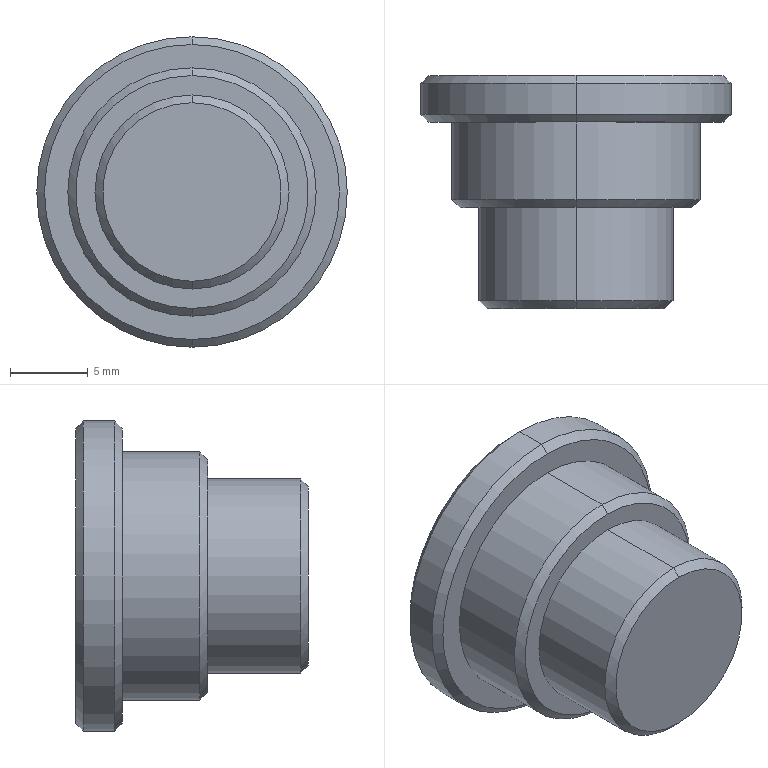Part | SolidWorks | features Chamfer 1, Revolution 1 | 1 solid | 18 faces | box 20 x 15 x 20 mm | volume 2820 mm3 | cone 8 | cylinder 6 | plane 4 | commonest cylinder face diameters 12.5 x2 16 x2 20 x2
STEP:
#1=CARTESIAN_POINT('',(82.463,-33.25,9.5));
#2=VERTEX_POINT('',#1);
#3=CARTESIAN_POINT('',(82.463,-33.25,-9.5));
#4=VERTEX_POINT('',#3);
#5=CARTESIAN_POINT('',(82.463,-33.25,0.));
#6=DIRECTION('',(0.,1.,0.));
#7=DIRECTION('',(0.,0.,1.));
#8=AXIS2_PLACEMENT_3D('',#5,#6,#7);
#9=CIRCLE('',#8,9.5);
#10=EDGE_CURVE('',#2,#4,#9,.T.);
#11=ORIENTED_EDGE('',*,*,#10,.F.);
#12=CARTESIAN_POINT('',(82.463,-33.75,10.));
#13=VERTEX_POINT('',#12);
#14=CARTESIAN_POINT('',(82.463,-33.75,10.));
#15=DIRECTION('',(0.,-0.7071,0.7071));
#16=VECTOR('',#15,1000.);
#17=LINE('',#14,#16);
#18=EDGE_CURVE('',#2,#13,#17,.T.);
#19=ORIENTED_EDGE('',*,*,#18,.T.);
#20=CARTESIAN_POINT('',(82.463,-33.75,-10.));
#21=VERTEX_POINT('',#20);
#22=CARTESIAN_POINT('',(82.463,-33.75,0.));
#23=DIRECTION('',(0.,-1.,0.));
#24=DIRECTION('',(0.,0.,1.));
#25=AXIS2_PLACEMENT_3D('',#22,#23,#24);
#26=CIRCLE('',#25,10.);
#27=EDGE_CURVE('',#21,#13,#26,.T.);
#28=ORIENTED_EDGE('',*,*,#27,.F.);
#29=CARTESIAN_POINT('',(82.463,-33.75,-10.));
#30=DIRECTION('',(0.,-0.7071,-0.7071));
#31=VECTOR('',#30,1000.);
#32=LINE('',#29,#31);
#33=EDGE_CURVE('',#4,#21,#32,.T.);
#34=ORIENTED_EDGE('',*,*,#33,.F.);
#35=EDGE_LOOP('',(#11,#19,#28,#34));
#36=FACE_OUTER_BOUND('',#35,.T.);
#37=CARTESIAN_POINT('',(82.463,-33.75,0.));
#38=DIRECTION('',(0.,-1.,0.));
#39=DIRECTION('',(0.,0.,-1.));
#40=AXIS2_PLACEMENT_3D('',#37,#38,#39);
#41=CONICAL_SURFACE('',#40,10.,0.7854);
#42=ADVANCED_FACE('',(#36),#41,.T.);
#43=CARTESIAN_POINT('',(82.463,-36.25,-9.5));
#44=VERTEX_POINT('',#43);
#45=CARTESIAN_POINT('',(82.463,-36.25,9.5));
#46=VERTEX_POINT('',#45);
#47=CARTESIAN_POINT('',(82.463,-36.25,0.));
#48=DIRECTION('',(0.,-1.,0.));
#49=DIRECTION('',(0.,0.,-1.));
#50=AXIS2_PLACEMENT_3D('',#47,#48,#49);
#51=CIRCLE('',#50,9.5);
#52=EDGE_CURVE('',#44,#46,#51,.T.);
#53=ORIENTED_EDGE('',*,*,#52,.F.);
#54=CARTESIAN_POINT('',(82.463,-35.75,-10.));
#55=VERTEX_POINT('',#54);
#56=CARTESIAN_POINT('',(82.463,-36.25,-9.5));
#57=DIRECTION('',(0.,0.7071,-0.7071));
#58=VECTOR('',#57,1000.);
#59=LINE('',#56,#58);
#60=EDGE_CURVE('',#44,#55,#59,.T.);
#61=ORIENTED_EDGE('',*,*,#60,.T.);
#62=CARTESIAN_POINT('',(82.463,-35.75,10.));
#63=VERTEX_POINT('',#62);
#64=CARTESIAN_POINT('',(82.463,-35.75,0.));
#65=DIRECTION('',(0.,1.,0.));
#66=DIRECTION('',(0.,0.,-1.));
#67=AXIS2_PLACEMENT_3D('',#64,#65,#66);
#68=CIRCLE('',#67,10.);
#69=EDGE_CURVE('',#63,#55,#68,.T.);
#70=ORIENTED_EDGE('',*,*,#69,.F.);
#71=CARTESIAN_POINT('',(82.463,-36.25,9.5));
#72=DIRECTION('',(0.,0.7071,0.7071));
#73=VECTOR('',#72,1000.);
#74=LINE('',#71,#73);
#75=EDGE_CURVE('',#46,#63,#74,.T.);
#76=ORIENTED_EDGE('',*,*,#75,.F.);
#77=EDGE_LOOP('',(#53,#61,#70,#76));
#78=FACE_OUTER_BOUND('',#77,.T.);
#79=CARTESIAN_POINT('',(82.463,-36.25,0.));
#80=DIRECTION('',(0.,1.,0.));
#81=DIRECTION('',(0.,0.,1.));
#82=AXIS2_PLACEMENT_3D('',#79,#80,#81);
#83=CONICAL_SURFACE('',#82,9.5,0.7854);
#84=ADVANCED_FACE('',(#78),#83,.T.);
#85=CARTESIAN_POINT('',(82.463,-41.75,-7.5));
#86=VERTEX_POINT('',#85);
#87=CARTESIAN_POINT('',(82.463,-41.75,7.5));
#88=VERTEX_POINT('',#87);
#89=CARTESIAN_POINT('',(82.463,-41.75,0.));
#90=DIRECTION('',(0.,-1.,0.));
#91=DIRECTION('',(0.,0.,-1.));
#92=AXIS2_PLACEMENT_3D('',#89,#90,#91);
#93=CIRCLE('',#92,7.5);
#94=EDGE_CURVE('',#86,#88,#93,.T.);
#95=ORIENTED_EDGE('',*,*,#94,.F.);
#96=CARTESIAN_POINT('',(82.463,-41.25,-8.));
#97=VERTEX_POINT('',#96);
#98=CARTESIAN_POINT('',(82.463,-41.75,-7.5));
#99=DIRECTION('',(0.,0.7071,-0.7071));
#100=VECTOR('',#99,1000.);
#101=LINE('',#98,#100);
#102=EDGE_CURVE('',#86,#97,#101,.T.);
#103=ORIENTED_EDGE('',*,*,#102,.T.);
#104=CARTESIAN_POINT('',(82.463,-41.25,8.));
#105=VERTEX_POINT('',#104);
#106=CARTESIAN_POINT('',(82.463,-41.25,0.));
#107=DIRECTION('',(0.,1.,0.));
#108=DIRECTION('',(0.,0.,-1.));
#109=AXIS2_PLACEMENT_3D('',#106,#107,#108);
#110=CIRCLE('',#109,8.);
#111=EDGE_CURVE('',#105,#97,#110,.T.);
#112=ORIENTED_EDGE('',*,*,#111,.F.);
#113=CARTESIAN_POINT('',(82.463,-41.75,7.5));
#114=DIRECTION('',(0.,0.7071,0.7071));
#115=VECTOR('',#114,1000.);
#116=LINE('',#113,#115);
#117=EDGE_CURVE('',#88,#105,#116,.T.);
#118=ORIENTED_EDGE('',*,*,#117,.F.);
#119=EDGE_LOOP('',(#95,#103,#112,#118));
#120=FACE_OUTER_BOUND('',#119,.T.);
#121=CARTESIAN_POINT('',(82.463,-41.75,0.));
#122=DIRECTION('',(0.,1.,0.));
#123=DIRECTION('',(0.,0.,1.));
#124=AXIS2_PLACEMENT_3D('',#121,#122,#123);
#125=CONICAL_SURFACE('',#124,7.5,0.7854);
#126=ADVANCED_FACE('',(#120),#125,.T.);
#127=CARTESIAN_POINT('',(82.463,-48.25,-5.75));
#128=VERTEX_POINT('',#127);
#129=CARTESIAN_POINT('',(82.463,-48.25,5.75));
#130=VERTEX_POINT('',#129);
#131=CARTESIAN_POINT('',(82.463,-48.25,0.));
#132=DIRECTION('',(0.,-1.,0.));
#133=DIRECTION('',(0.,0.,-1.));
#134=AXIS2_PLACEMENT_3D('',#131,#132,#133);
#135=CIRCLE('',#134,5.75);
#136=EDGE_CURVE('',#128,#130,#135,.T.);
#137=ORIENTED_EDGE('',*,*,#136,.F.);
#138=CARTESIAN_POINT('',(82.463,-47.75,-6.25));
#139=VERTEX_POINT('',#138);
#140=CARTESIAN_POINT('',(82.463,-48.25,-5.75));
#141=DIRECTION('',(0.,0.7071,-0.7071));
#142=VECTOR('',#141,1000.);
#143=LINE('',#140,#142);
#144=EDGE_CURVE('',#128,#139,#143,.T.);
#145=ORIENTED_EDGE('',*,*,#144,.T.);
#146=CARTESIAN_POINT('',(82.463,-47.75,6.25));
#147=VERTEX_POINT('',#146);
#148=CARTESIAN_POINT('',(82.463,-47.75,0.));
#149=DIRECTION('',(0.,1.,0.));
#150=DIRECTION('',(0.,0.,-1.));
#151=AXIS2_PLACEMENT_3D('',#148,#149,#150);
#152=CIRCLE('',#151,6.25);
#153=EDGE_CURVE('',#147,#139,#152,.T.);
#154=ORIENTED_EDGE('',*,*,#153,.F.);
#155=CARTESIAN_POINT('',(82.463,-48.25,5.75));
#156=DIRECTION('',(0.,0.7071,0.7071));
#157=VECTOR('',#156,1000.);
#158=LINE('',#155,#157);
#159=EDGE_CURVE('',#130,#147,#158,.T.);
#160=ORIENTED_EDGE('',*,*,#159,.F.);
#161=EDGE_LOOP('',(#137,#145,#154,#160));
#162=FACE_OUTER_BOUND('',#161,.T.);
#163=CARTESIAN_POINT('',(82.463,-48.25,0.));
#164=DIRECTION('',(0.,1.,0.));
#165=DIRECTION('',(0.,0.,1.));
#166=AXIS2_PLACEMENT_3D('',#163,#164,#165);
#167=CONICAL_SURFACE('',#166,5.75,0.7854);
#168=ADVANCED_FACE('',(#162),#167,.T.);
#169=ORIENTED_EDGE('',*,*,#27,.T.);
#170=CARTESIAN_POINT('',(82.463,-48.25,10.));
#171=DIRECTION('',(0.,-1.,0.));
#172=VECTOR('',#171,1000.);
#173=LINE('',#170,#172);
#174=EDGE_CURVE('',#13,#63,#173,.T.);
#175=ORIENTED_EDGE('',*,*,#174,.T.);
#176=ORIENTED_EDGE('',*,*,#69,.T.);
#177=CARTESIAN_POINT('',(82.463,-48.25,-10.));
#178=DIRECTION('',(0.,-1.,0.));
#179=VECTOR('',#178,1000.);
#180=LINE('',#177,#179);
#181=EDGE_CURVE('',#21,#55,#180,.T.);
#182=ORIENTED_EDGE('',*,*,#181,.F.);
#183=EDGE_LOOP('',(#169,#175,#176,#182));
#184=FACE_OUTER_BOUND('',#183,.T.);
#185=CARTESIAN_POINT('',(82.463,-48.25,0.));
#186=DIRECTION('',(0.,-1.,0.));
#187=DIRECTION('',(0.,0.,-1.));
#188=AXIS2_PLACEMENT_3D('',#185,#186,#187);
#189=CYLINDRICAL_SURFACE('',#188,10.);
#190=ADVANCED_FACE('',(#184),#189,.T.);
#191=CARTESIAN_POINT('',(82.463,-36.25,-8.));
#192=VERTEX_POINT('',#191);
#193=CARTESIAN_POINT('',(82.463,-36.25,8.));
#194=VERTEX_POINT('',#193);
#195=CARTESIAN_POINT('',(82.463,-36.25,0.));
#196=DIRECTION('',(0.,-1.,0.));
#197=DIRECTION('',(0.,0.,-1.));
#198=AXIS2_PLACEMENT_3D('',#195,#196,#197);
#199=CIRCLE('',#198,8.);
#200=EDGE_CURVE('',#192,#194,#199,.T.);
#201=ORIENTED_EDGE('',*,*,#200,.T.);
#202=CARTESIAN_POINT('',(82.463,-48.25,8.));
#203=DIRECTION('',(0.,-1.,0.));
#204=VECTOR('',#203,1000.);
#205=LINE('',#202,#204);
#206=EDGE_CURVE('',#194,#105,#205,.T.);
#207=ORIENTED_EDGE('',*,*,#206,.T.);
#208=ORIENTED_EDGE('',*,*,#111,.T.);
#209=CARTESIAN_POINT('',(82.463,-48.25,-8.));
#210=DIRECTION('',(0.,-1.,0.));
#211=VECTOR('',#210,1000.);
#212=LINE('',#209,#211);
#213=EDGE_CURVE('',#192,#97,#212,.T.);
#214=ORIENTED_EDGE('',*,*,#213,.F.);
#215=EDGE_LOOP('',(#201,#207,#208,#214));
#216=FACE_OUTER_BOUND('',#215,.T.);
#217=CARTESIAN_POINT('',(82.463,-48.25,0.));
#218=DIRECTION('',(0.,-1.,0.));
#219=DIRECTION('',(0.,0.,-1.));
#220=AXIS2_PLACEMENT_3D('',#217,#218,#219);
#221=CYLINDRICAL_SURFACE('',#220,8.);
#222=ADVANCED_FACE('',(#216),#221,.T.);
#223=CARTESIAN_POINT('',(82.463,-41.75,-6.25));
#224=VERTEX_POINT('',#223);
#225=CARTESIAN_POINT('',(82.463,-41.75,6.25));
#226=VERTEX_POINT('',#225);
#227=CARTESIAN_POINT('',(82.463,-41.75,0.));
#228=DIRECTION('',(0.,-1.,0.));
#229=DIRECTION('',(0.,0.,-1.));
#230=AXIS2_PLACEMENT_3D('',#227,#228,#229);
#231=CIRCLE('',#230,6.25);
#232=EDGE_CURVE('',#224,#226,#231,.T.);
#233=ORIENTED_EDGE('',*,*,#232,.T.);
#234=CARTESIAN_POINT('',(82.463,-48.25,6.25));
#235=DIRECTION('',(0.,-1.,0.));
#236=VECTOR('',#235,1000.);
#237=LINE('',#234,#236);
#238=EDGE_CURVE('',#226,#147,#237,.T.);
#239=ORIENTED_EDGE('',*,*,#238,.T.);
#240=ORIENTED_EDGE('',*,*,#153,.T.);
#241=CARTESIAN_POINT('',(82.463,-48.25,-6.25));
#242=DIRECTION('',(0.,-1.,0.));
#243=VECTOR('',#242,1000.);
#244=LINE('',#241,#243);
#245=EDGE_CURVE('',#224,#139,#244,.T.);
#246=ORIENTED_EDGE('',*,*,#245,.F.);
#247=EDGE_LOOP('',(#233,#239,#240,#246));
#248=FACE_OUTER_BOUND('',#247,.T.);
#249=CARTESIAN_POINT('',(82.463,-48.25,0.));
#250=DIRECTION('',(0.,-1.,0.));
#251=DIRECTION('',(0.,0.,-1.));
#252=AXIS2_PLACEMENT_3D('',#249,#250,#251);
#253=CYLINDRICAL_SURFACE('',#252,6.25);
#254=ADVANCED_FACE('',(#248),#253,.T.);
#255=CARTESIAN_POINT('',(82.463,-48.25,0.));
#256=DIRECTION('',(0.,-1.,0.));
#257=DIRECTION('',(0.,0.,-1.));
#258=AXIS2_PLACEMENT_3D('',#255,#256,#257);
#259=CIRCLE('',#258,5.75);
#260=EDGE_CURVE('',#130,#128,#259,.T.);
#261=ORIENTED_EDGE('',*,*,#260,.T.);
#262=ORIENTED_EDGE('',*,*,#136,.T.);
#263=EDGE_LOOP('',(#261,#262));
#264=FACE_OUTER_BOUND('',#263,.T.);
#265=CARTESIAN_POINT('',(88.713,-48.25,0.));
#266=DIRECTION('',(0.,-1.,0.));
#267=DIRECTION('',(0.,0.,-1.));
#268=AXIS2_PLACEMENT_3D('',#265,#266,#267);
#269=PLANE('',#268);
#270=ADVANCED_FACE('',(#264),#269,.T.);
#271=ORIENTED_EDGE('',*,*,#238,.F.);
#272=CARTESIAN_POINT('',(82.463,-41.75,0.));
#273=DIRECTION('',(0.,-1.,0.));
#274=DIRECTION('',(0.,0.,-1.));
#275=AXIS2_PLACEMENT_3D('',#272,#273,#274);
#276=CIRCLE('',#275,6.25);
#277=EDGE_CURVE('',#226,#224,#276,.T.);
#278=ORIENTED_EDGE('',*,*,#277,.T.);
#279=ORIENTED_EDGE('',*,*,#245,.T.);
#280=CARTESIAN_POINT('',(82.463,-47.75,0.));
#281=DIRECTION('',(0.,1.,0.));
#282=DIRECTION('',(0.,0.,-1.));
#283=AXIS2_PLACEMENT_3D('',#280,#281,#282);
#284=CIRCLE('',#283,6.25);
#285=EDGE_CURVE('',#139,#147,#284,.T.);
#286=ORIENTED_EDGE('',*,*,#285,.T.);
#287=EDGE_LOOP('',(#271,#278,#279,#286));
#288=FACE_OUTER_BOUND('',#287,.T.);
#289=CARTESIAN_POINT('',(82.463,-48.25,0.));
#290=DIRECTION('',(0.,-1.,0.));
#291=DIRECTION('',(0.,0.,-1.));
#292=AXIS2_PLACEMENT_3D('',#289,#290,#291);
#293=CYLINDRICAL_SURFACE('',#292,6.25);
#294=ADVANCED_FACE('',(#288),#293,.T.);
#295=CARTESIAN_POINT('',(82.463,-41.75,0.));
#296=DIRECTION('',(0.,-1.,0.));
#297=DIRECTION('',(0.,0.,-1.));
#298=AXIS2_PLACEMENT_3D('',#295,#296,#297);
#299=CIRCLE('',#298,7.5);
#300=EDGE_CURVE('',#88,#86,#299,.T.);
#301=ORIENTED_EDGE('',*,*,#300,.T.);
#302=ORIENTED_EDGE('',*,*,#94,.T.);
#303=EDGE_LOOP('',(#301,#302));
#304=FACE_OUTER_BOUND('',#303,.T.);
#305=ORIENTED_EDGE('',*,*,#232,.F.);
#306=ORIENTED_EDGE('',*,*,#277,.F.);
#307=EDGE_LOOP('',(#305,#306));
#308=FACE_BOUND('',#307,.T.);
#309=CARTESIAN_POINT('',(88.713,-41.75,0.));
#310=DIRECTION('',(0.,-1.,0.));
#311=DIRECTION('',(0.,0.,-1.));
#312=AXIS2_PLACEMENT_3D('',#309,#310,#311);
#313=PLANE('',#312);
#314=ADVANCED_FACE('',(#304,#308),#313,.T.);
#315=ORIENTED_EDGE('',*,*,#206,.F.);
#316=CARTESIAN_POINT('',(82.463,-36.25,0.));
#317=DIRECTION('',(0.,-1.,0.));
#318=DIRECTION('',(0.,0.,-1.));
#319=AXIS2_PLACEMENT_3D('',#316,#317,#318);
#320=CIRCLE('',#319,8.);
#321=EDGE_CURVE('',#194,#192,#320,.T.);
#322=ORIENTED_EDGE('',*,*,#321,.T.);
#323=ORIENTED_EDGE('',*,*,#213,.T.);
#324=CARTESIAN_POINT('',(82.463,-41.25,0.));
#325=DIRECTION('',(0.,1.,0.));
#326=DIRECTION('',(0.,0.,-1.));
#327=AXIS2_PLACEMENT_3D('',#324,#325,#326);
#328=CIRCLE('',#327,8.);
#329=EDGE_CURVE('',#97,#105,#328,.T.);
#330=ORIENTED_EDGE('',*,*,#329,.T.);
#331=EDGE_LOOP('',(#315,#322,#323,#330));
#332=FACE_OUTER_BOUND('',#331,.T.);
#333=CARTESIAN_POINT('',(82.463,-48.25,0.));
#334=DIRECTION('',(0.,-1.,0.));
#335=DIRECTION('',(0.,0.,-1.));
#336=AXIS2_PLACEMENT_3D('',#333,#334,#335);
#337=CYLINDRICAL_SURFACE('',#336,8.);
#338=ADVANCED_FACE('',(#332),#337,.T.);
#339=CARTESIAN_POINT('',(82.463,-36.25,0.));
#340=DIRECTION('',(0.,-1.,0.));
#341=DIRECTION('',(0.,0.,-1.));
#342=AXIS2_PLACEMENT_3D('',#339,#340,#341);
#343=CIRCLE('',#342,9.5);
#344=EDGE_CURVE('',#46,#44,#343,.T.);
#345=ORIENTED_EDGE('',*,*,#344,.T.);
#346=ORIENTED_EDGE('',*,*,#52,.T.);
#347=EDGE_LOOP('',(#345,#346));
#348=FACE_OUTER_BOUND('',#347,.T.);
#349=ORIENTED_EDGE('',*,*,#200,.F.);
#350=ORIENTED_EDGE('',*,*,#321,.F.);
#351=EDGE_LOOP('',(#349,#350));
#352=FACE_BOUND('',#351,.T.);
#353=CARTESIAN_POINT('',(90.463,-36.25,0.));
#354=DIRECTION('',(0.,-1.,0.));
#355=DIRECTION('',(0.,0.,-1.));
#356=AXIS2_PLACEMENT_3D('',#353,#354,#355);
#357=PLANE('',#356);
#358=ADVANCED_FACE('',(#348,#352),#357,.T.);
#359=ORIENTED_EDGE('',*,*,#174,.F.);
#360=CARTESIAN_POINT('',(82.463,-33.75,0.));
#361=DIRECTION('',(0.,-1.,0.));
#362=DIRECTION('',(0.,0.,1.));
#363=AXIS2_PLACEMENT_3D('',#360,#361,#362);
#364=CIRCLE('',#363,10.);
#365=EDGE_CURVE('',#13,#21,#364,.T.);
#366=ORIENTED_EDGE('',*,*,#365,.T.);
#367=ORIENTED_EDGE('',*,*,#181,.T.);
#368=CARTESIAN_POINT('',(82.463,-35.75,0.));
#369=DIRECTION('',(0.,1.,0.));
#370=DIRECTION('',(0.,0.,-1.));
#371=AXIS2_PLACEMENT_3D('',#368,#369,#370);
#372=CIRCLE('',#371,10.);
#373=EDGE_CURVE('',#55,#63,#372,.T.);
#374=ORIENTED_EDGE('',*,*,#373,.T.);
#375=EDGE_LOOP('',(#359,#366,#367,#374));
#376=FACE_OUTER_BOUND('',#375,.T.);
#377=CARTESIAN_POINT('',(82.463,-48.25,0.));
#378=DIRECTION('',(0.,-1.,0.));
#379=DIRECTION('',(0.,0.,-1.));
#380=AXIS2_PLACEMENT_3D('',#377,#378,#379);
#381=CYLINDRICAL_SURFACE('',#380,10.);
#382=ADVANCED_FACE('',(#376),#381,.T.);
#383=CARTESIAN_POINT('',(82.463,-33.25,0.));
#384=DIRECTION('',(0.,1.,0.));
#385=DIRECTION('',(0.,0.,1.));
#386=AXIS2_PLACEMENT_3D('',#383,#384,#385);
#387=CIRCLE('',#386,9.5);
#388=EDGE_CURVE('',#4,#2,#387,.T.);
#389=ORIENTED_EDGE('',*,*,#388,.T.);
#390=ORIENTED_EDGE('',*,*,#10,.T.);
#391=EDGE_LOOP('',(#389,#390));
#392=FACE_OUTER_BOUND('',#391,.T.);
#393=CARTESIAN_POINT('',(92.463,-33.25,0.));
#394=DIRECTION('',(0.,1.,0.));
#395=DIRECTION('',(0.,0.,1.));
#396=AXIS2_PLACEMENT_3D('',#393,#394,#395);
#397=PLANE('',#396);
#398=ADVANCED_FACE('',(#392),#397,.T.);
#399=ORIENTED_EDGE('',*,*,#144,.F.);
#400=ORIENTED_EDGE('',*,*,#260,.F.);
#401=ORIENTED_EDGE('',*,*,#159,.T.);
#402=ORIENTED_EDGE('',*,*,#285,.F.);
#403=EDGE_LOOP('',(#399,#400,#401,#402));
#404=FACE_OUTER_BOUND('',#403,.T.);
#405=CARTESIAN_POINT('',(82.463,-48.25,0.));
#406=DIRECTION('',(0.,1.,0.));
#407=DIRECTION('',(0.,0.,1.));
#408=AXIS2_PLACEMENT_3D('',#405,#406,#407);
#409=CONICAL_SURFACE('',#408,5.75,0.7854);
#410=ADVANCED_FACE('',(#404),#409,.T.);
#411=ORIENTED_EDGE('',*,*,#102,.F.);
#412=ORIENTED_EDGE('',*,*,#300,.F.);
#413=ORIENTED_EDGE('',*,*,#117,.T.);
#414=ORIENTED_EDGE('',*,*,#329,.F.);
#415=EDGE_LOOP('',(#411,#412,#413,#414));
#416=FACE_OUTER_BOUND('',#415,.T.);
#417=CARTESIAN_POINT('',(82.463,-41.75,0.));
#418=DIRECTION('',(0.,1.,0.));
#419=DIRECTION('',(0.,0.,1.));
#420=AXIS2_PLACEMENT_3D('',#417,#418,#419);
#421=CONICAL_SURFACE('',#420,7.5,0.7854);
#422=ADVANCED_FACE('',(#416),#421,.T.);
#423=ORIENTED_EDGE('',*,*,#60,.F.);
#424=ORIENTED_EDGE('',*,*,#344,.F.);
#425=ORIENTED_EDGE('',*,*,#75,.T.);
#426=ORIENTED_EDGE('',*,*,#373,.F.);
#427=EDGE_LOOP('',(#423,#424,#425,#426));
#428=FACE_OUTER_BOUND('',#427,.T.);
#429=CARTESIAN_POINT('',(82.463,-36.25,0.));
#430=DIRECTION('',(0.,1.,0.));
#431=DIRECTION('',(0.,0.,1.));
#432=AXIS2_PLACEMENT_3D('',#429,#430,#431);
#433=CONICAL_SURFACE('',#432,9.5,0.7854);
#434=ADVANCED_FACE('',(#428),#433,.T.);
#435=ORIENTED_EDGE('',*,*,#18,.F.);
#436=ORIENTED_EDGE('',*,*,#388,.F.);
#437=ORIENTED_EDGE('',*,*,#33,.T.);
#438=ORIENTED_EDGE('',*,*,#365,.F.);
#439=EDGE_LOOP('',(#435,#436,#437,#438));
#440=FACE_OUTER_BOUND('',#439,.T.);
#441=CARTESIAN_POINT('',(82.463,-33.75,0.));
#442=DIRECTION('',(0.,-1.,0.));
#443=DIRECTION('',(0.,0.,-1.));
#444=AXIS2_PLACEMENT_3D('',#441,#442,#443);
#445=CONICAL_SURFACE('',#444,10.,0.7854);
#446=ADVANCED_FACE('',(#440),#445,.T.);
#447=CLOSED_SHELL('',(#42,#84,#126,#168,#190,#222,#254,#270,#294,#314,#338,#358,#382,#398,#410,#422,#434,#446));
#448=MANIFOLD_SOLID_BREP('',#447);
#449=CARTESIAN_POINT('',(0.,0.,0.));
#450=DIRECTION('',(0.,0.,1.));
#451=DIRECTION('',(1.,0.,0.));
#452=AXIS2_PLACEMENT_3D('',#449,#450,#451);
#453=(LENGTH_UNIT()NAMED_UNIT(*)SI_UNIT(.MILLI.,.METRE.));
#454=UNCERTAINTY_MEASURE_WITH_UNIT(LENGTH_MEASURE(0.00001),#453,'','');
#455=(NAMED_UNIT(*)PLANE_ANGLE_UNIT()SI_UNIT($,.RADIAN.));
#456=(NAMED_UNIT(*)SI_UNIT($,.STERADIAN.)SOLID_ANGLE_UNIT());
#457=(GEOMETRIC_REPRESENTATION_CONTEXT(3)GLOBAL_UNCERTAINTY_ASSIGNED_CONTEXT((#454))GLOBAL_UNIT_ASSIGNED_CONTEXT((#453,#455,#456))REPRESENTATION_CONTEXT('',''));
#458=ADVANCED_BREP_SHAPE_REPRESENTATION('',(#448,#452),#457);